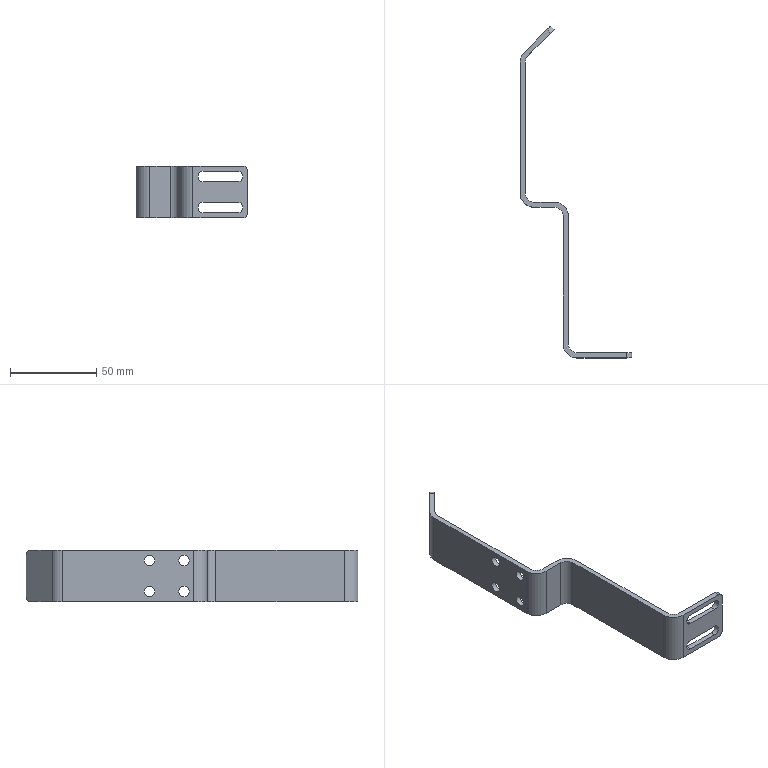Part | NX | features BREP 1 | 1 solid | 38 faces | box 65 x 192.678 x 30 mm | volume 21438 mm3 | cylinder 20 | plane 18 | commonest cylinder face diameters 6 x12 10 x4 16 x4
STEP:
#1=CARTESIAN_POINT('',(3.,82.5,30.));
#2=VERTEX_POINT('',#1);
#3=CARTESIAN_POINT('',(3.,82.5,0.));
#4=VERTEX_POINT('',#3);
#5=CARTESIAN_POINT('',(3.,82.5,30.));
#6=DIRECTION('',(0.,0.,-1.));
#7=VECTOR('',#6,1000.);
#8=LINE('',#5,#7);
#9=EDGE_CURVE('',#2,#4,#8,.T.);
#10=ORIENTED_EDGE('',*,*,#9,.F.);
#11=CARTESIAN_POINT('',(3.,8.,30.));
#12=VERTEX_POINT('',#11);
#13=CARTESIAN_POINT('',(3.,0.,30.));
#14=DIRECTION('',(0.,1.,0.));
#15=VECTOR('',#14,1000.);
#16=LINE('',#13,#15);
#17=EDGE_CURVE('',#12,#2,#16,.T.);
#18=ORIENTED_EDGE('',*,*,#17,.F.);
#19=CARTESIAN_POINT('',(3.,8.,0.));
#20=VERTEX_POINT('',#19);
#21=CARTESIAN_POINT('',(3.,8.,30.));
#22=DIRECTION('',(0.,0.,1.));
#23=VECTOR('',#22,1000.);
#24=LINE('',#21,#23);
#25=EDGE_CURVE('',#20,#12,#24,.T.);
#26=ORIENTED_EDGE('',*,*,#25,.F.);
#27=CARTESIAN_POINT('',(3.,0.,0.));
#28=DIRECTION('',(0.,-1.,0.));
#29=VECTOR('',#28,1000.);
#30=LINE('',#27,#29);
#31=EDGE_CURVE('',#4,#20,#30,.T.);
#32=ORIENTED_EDGE('',*,*,#31,.F.);
#33=EDGE_LOOP('',(#10,#18,#26,#32));
#34=FACE_BOUND('',#33,.T.);
#35=CARTESIAN_POINT('',(3.,0.,30.));
#36=DIRECTION('',(-1.,0.,0.));
#37=DIRECTION('',(0.,0.,-1.));
#38=AXIS2_PLACEMENT_3D('',#35,#36,#37);
#39=PLANE('',#38);
#40=ADVANCED_FACE('',(#34),#39,.F.);
#41=ORIENTED_EDGE('',*,*,#31,.T.);
#42=CARTESIAN_POINT('',(8.,3.,0.));
#43=VERTEX_POINT('',#42);
#44=CARTESIAN_POINT('',(8.,8.,0.));
#45=DIRECTION('',(0.,0.,1.));
#46=DIRECTION('',(-1.,0.,0.));
#47=AXIS2_PLACEMENT_3D('',#44,#45,#46);
#48=CIRCLE('',#47,5.);
#49=EDGE_CURVE('',#20,#43,#48,.T.);
#50=ORIENTED_EDGE('',*,*,#49,.T.);
#51=CARTESIAN_POINT('',(37.,3.,0.));
#52=VERTEX_POINT('',#51);
#53=CARTESIAN_POINT('',(40.,3.,0.));
#54=DIRECTION('',(1.,0.,0.));
#55=VECTOR('',#54,1000.);
#56=LINE('',#53,#55);
#57=EDGE_CURVE('',#43,#52,#56,.T.);
#58=ORIENTED_EDGE('',*,*,#57,.T.);
#59=CARTESIAN_POINT('',(37.,0.,0.));
#60=VERTEX_POINT('',#59);
#61=CARTESIAN_POINT('',(37.,8.,0.));
#62=DIRECTION('',(0.,-1.,0.));
#63=VECTOR('',#62,1000.);
#64=LINE('',#61,#63);
#65=EDGE_CURVE('',#52,#60,#64,.T.);
#66=ORIENTED_EDGE('',*,*,#65,.T.);
#67=CARTESIAN_POINT('',(8.,0.,0.));
#68=VERTEX_POINT('',#67);
#69=CARTESIAN_POINT('',(3.,0.,0.));
#70=DIRECTION('',(-1.,0.,0.));
#71=VECTOR('',#70,1000.);
#72=LINE('',#69,#71);
#73=EDGE_CURVE('',#60,#68,#72,.T.);
#74=ORIENTED_EDGE('',*,*,#73,.T.);
#75=CARTESIAN_POINT('',(0.,8.,0.));
#76=VERTEX_POINT('',#75);
#77=CARTESIAN_POINT('',(8.,8.,0.));
#78=DIRECTION('',(0.,0.,-1.));
#79=DIRECTION('',(-1.,0.,0.));
#80=AXIS2_PLACEMENT_3D('',#77,#78,#79);
#81=CIRCLE('',#80,8.);
#82=EDGE_CURVE('',#68,#76,#81,.T.);
#83=ORIENTED_EDGE('',*,*,#82,.T.);
#84=CARTESIAN_POINT('',(0.,82.5,0.));
#85=VERTEX_POINT('',#84);
#86=CARTESIAN_POINT('',(0.,90.5,0.));
#87=DIRECTION('',(0.,1.,0.));
#88=VECTOR('',#87,1000.);
#89=LINE('',#86,#88);
#90=EDGE_CURVE('',#76,#85,#89,.T.);
#91=ORIENTED_EDGE('',*,*,#90,.T.);
#92=CARTESIAN_POINT('',(-5.,87.5,0.));
#93=VERTEX_POINT('',#92);
#94=CARTESIAN_POINT('',(-5.,82.5,0.));
#95=DIRECTION('',(0.,0.,1.));
#96=DIRECTION('',(-1.,0.,0.));
#97=AXIS2_PLACEMENT_3D('',#94,#95,#96);
#98=CIRCLE('',#97,5.);
#99=EDGE_CURVE('',#85,#93,#98,.T.);
#100=ORIENTED_EDGE('',*,*,#99,.T.);
#101=CARTESIAN_POINT('',(-17.,87.5,0.));
#102=VERTEX_POINT('',#101);
#103=CARTESIAN_POINT('',(-22.,87.5,0.));
#104=DIRECTION('',(-1.,0.,0.));
#105=VECTOR('',#104,1000.);
#106=LINE('',#103,#105);
#107=EDGE_CURVE('',#93,#102,#106,.T.);
#108=ORIENTED_EDGE('',*,*,#107,.T.);
#109=CARTESIAN_POINT('',(-25.,95.5,0.));
#110=VERTEX_POINT('',#109);
#111=CARTESIAN_POINT('',(-17.,95.5,0.));
#112=DIRECTION('',(0.,0.,-1.));
#113=DIRECTION('',(-1.,0.,0.));
#114=AXIS2_PLACEMENT_3D('',#111,#112,#113);
#115=CIRCLE('',#114,8.);
#116=EDGE_CURVE('',#102,#110,#115,.T.);
#117=ORIENTED_EDGE('',*,*,#116,.T.);
#118=CARTESIAN_POINT('',(-25.,171.686,0.));
#119=VERTEX_POINT('',#118);
#120=CARTESIAN_POINT('',(-25.,175.222,0.));
#121=DIRECTION('',(0.,1.,0.));
#122=VECTOR('',#121,1000.);
#123=LINE('',#120,#122);
#124=EDGE_CURVE('',#110,#119,#123,.T.);
#125=ORIENTED_EDGE('',*,*,#124,.T.);
#126=CARTESIAN_POINT('',(-22.657,177.343,0.));
#127=VERTEX_POINT('',#126);
#128=CARTESIAN_POINT('',(-17.,171.686,0.));
#129=DIRECTION('',(0.,0.,-1.));
#130=DIRECTION('',(-1.,0.,0.));
#131=AXIS2_PLACEMENT_3D('',#128,#129,#130);
#132=CIRCLE('',#131,8.);
#133=EDGE_CURVE('',#119,#127,#132,.T.);
#134=ORIENTED_EDGE('',*,*,#133,.T.);
#135=CARTESIAN_POINT('',(-9.444,190.556,0.));
#136=VERTEX_POINT('',#135);
#137=CARTESIAN_POINT('',(-9.444,190.556,0.));
#138=DIRECTION('',(-0.7071,-0.7071,0.));
#139=VECTOR('',#138,1000.);
#140=LINE('',#137,#139);
#141=EDGE_CURVE('',#136,#127,#140,.T.);
#142=ORIENTED_EDGE('',*,*,#141,.F.);
#143=CARTESIAN_POINT('',(-7.322,188.435,0.));
#144=VERTEX_POINT('',#143);
#145=CARTESIAN_POINT('',(-7.322,188.435,0.));
#146=DIRECTION('',(-0.7071,0.7071,0.));
#147=VECTOR('',#146,1000.);
#148=LINE('',#145,#147);
#149=EDGE_CURVE('',#144,#136,#148,.T.);
#150=ORIENTED_EDGE('',*,*,#149,.F.);
#151=CARTESIAN_POINT('',(-20.536,175.222,0.));
#152=VERTEX_POINT('',#151);
#153=CARTESIAN_POINT('',(-22.879,172.879,0.));
#154=DIRECTION('',(-0.7071,-0.7071,0.));
#155=VECTOR('',#154,1000.);
#156=LINE('',#153,#155);
#157=EDGE_CURVE('',#144,#152,#156,.T.);
#158=ORIENTED_EDGE('',*,*,#157,.T.);
#159=CARTESIAN_POINT('',(-22.,171.686,0.));
#160=VERTEX_POINT('',#159);
#161=CARTESIAN_POINT('',(-17.,171.686,0.));
#162=DIRECTION('',(0.,0.,1.));
#163=DIRECTION('',(-1.,0.,0.));
#164=AXIS2_PLACEMENT_3D('',#161,#162,#163);
#165=CIRCLE('',#164,5.);
#166=EDGE_CURVE('',#152,#160,#165,.T.);
#167=ORIENTED_EDGE('',*,*,#166,.T.);
#168=CARTESIAN_POINT('',(-22.,95.5,0.));
#169=VERTEX_POINT('',#168);
#170=CARTESIAN_POINT('',(-22.,87.5,0.));
#171=DIRECTION('',(0.,-1.,0.));
#172=VECTOR('',#171,1000.);
#173=LINE('',#170,#172);
#174=EDGE_CURVE('',#160,#169,#173,.T.);
#175=ORIENTED_EDGE('',*,*,#174,.T.);
#176=CARTESIAN_POINT('',(-17.,90.5,0.));
#177=VERTEX_POINT('',#176);
#178=CARTESIAN_POINT('',(-17.,95.5,0.));
#179=DIRECTION('',(0.,0.,1.));
#180=DIRECTION('',(-1.,0.,0.));
#181=AXIS2_PLACEMENT_3D('',#178,#179,#180);
#182=CIRCLE('',#181,5.);
#183=EDGE_CURVE('',#169,#177,#182,.T.);
#184=ORIENTED_EDGE('',*,*,#183,.T.);
#185=CARTESIAN_POINT('',(-5.,90.5,0.));
#186=VERTEX_POINT('',#185);
#187=CARTESIAN_POINT('',(0.,90.5,0.));
#188=DIRECTION('',(1.,0.,0.));
#189=VECTOR('',#188,1000.);
#190=LINE('',#187,#189);
#191=EDGE_CURVE('',#177,#186,#190,.T.);
#192=ORIENTED_EDGE('',*,*,#191,.T.);
#193=CARTESIAN_POINT('',(-5.,82.5,0.));
#194=DIRECTION('',(0.,0.,1.));
#195=DIRECTION('',(-1.,0.,0.));
#196=AXIS2_PLACEMENT_3D('',#193,#194,#195);
#197=CIRCLE('',#196,8.);
#198=EDGE_CURVE('',#4,#186,#197,.T.);
#199=ORIENTED_EDGE('',*,*,#198,.F.);
#200=EDGE_LOOP('',(#41,#50,#58,#66,#74,#83,#91,#100,#108,#117,#125,#134,#142,#150,#158,#167,#175,#184,#192,#199));
#201=FACE_BOUND('',#200,.T.);
#202=CARTESIAN_POINT('',(-5.,90.5,0.));
#203=DIRECTION('',(0.,0.,-1.));
#204=DIRECTION('',(1.,0.,0.));
#205=AXIS2_PLACEMENT_3D('',#202,#203,#204);
#206=PLANE('',#205);
#207=ADVANCED_FACE('',(#201),#206,.T.);
#208=CARTESIAN_POINT('',(-5.,90.5,30.));
#209=VERTEX_POINT('',#208);
#210=CARTESIAN_POINT('',(-5.,82.5,30.));
#211=DIRECTION('',(0.,0.,-1.));
#212=DIRECTION('',(-1.,0.,0.));
#213=AXIS2_PLACEMENT_3D('',#210,#211,#212);
#214=CIRCLE('',#213,8.);
#215=EDGE_CURVE('',#209,#2,#214,.T.);
#216=ORIENTED_EDGE('',*,*,#215,.T.);
#217=ORIENTED_EDGE('',*,*,#9,.T.);
#218=ORIENTED_EDGE('',*,*,#198,.T.);
#219=CARTESIAN_POINT('',(-5.,90.5,30.));
#220=DIRECTION('',(0.,0.,1.));
#221=VECTOR('',#220,1000.);
#222=LINE('',#219,#221);
#223=EDGE_CURVE('',#186,#209,#222,.T.);
#224=ORIENTED_EDGE('',*,*,#223,.T.);
#225=EDGE_LOOP('',(#216,#217,#218,#224));
#226=FACE_BOUND('',#225,.T.);
#227=CARTESIAN_POINT('',(-5.,82.5,30.));
#228=DIRECTION('',(0.,0.,-1.));
#229=DIRECTION('',(1.,0.,0.));
#230=AXIS2_PLACEMENT_3D('',#227,#228,#229);
#231=CYLINDRICAL_SURFACE('',#230,8.);
#232=ADVANCED_FACE('',(#226),#231,.T.);
#233=ORIENTED_EDGE('',*,*,#17,.T.);
#234=ORIENTED_EDGE('',*,*,#215,.F.);
#235=CARTESIAN_POINT('',(-17.,90.5,30.));
#236=VERTEX_POINT('',#235);
#237=CARTESIAN_POINT('',(0.,90.5,30.));
#238=DIRECTION('',(-1.,0.,0.));
#239=VECTOR('',#238,1000.);
#240=LINE('',#237,#239);
#241=EDGE_CURVE('',#209,#236,#240,.T.);
#242=ORIENTED_EDGE('',*,*,#241,.T.);
#243=CARTESIAN_POINT('',(-22.,95.5,30.));
#244=VERTEX_POINT('',#243);
#245=CARTESIAN_POINT('',(-17.,95.5,30.));
#246=DIRECTION('',(0.,0.,-1.));
#247=DIRECTION('',(-1.,0.,0.));
#248=AXIS2_PLACEMENT_3D('',#245,#246,#247);
#249=CIRCLE('',#248,5.);
#250=EDGE_CURVE('',#236,#244,#249,.T.);
#251=ORIENTED_EDGE('',*,*,#250,.T.);
#252=CARTESIAN_POINT('',(-22.,171.686,30.));
#253=VERTEX_POINT('',#252);
#254=CARTESIAN_POINT('',(-22.,87.5,30.));
#255=DIRECTION('',(0.,1.,0.));
#256=VECTOR('',#255,1000.);
#257=LINE('',#254,#256);
#258=EDGE_CURVE('',#244,#253,#257,.T.);
#259=ORIENTED_EDGE('',*,*,#258,.T.);
#260=CARTESIAN_POINT('',(-20.536,175.222,30.));
#261=VERTEX_POINT('',#260);
#262=CARTESIAN_POINT('',(-17.,171.686,30.));
#263=DIRECTION('',(0.,0.,-1.));
#264=DIRECTION('',(-1.,0.,0.));
#265=AXIS2_PLACEMENT_3D('',#262,#263,#264);
#266=CIRCLE('',#265,5.);
#267=EDGE_CURVE('',#253,#261,#266,.T.);
#268=ORIENTED_EDGE('',*,*,#267,.T.);
#269=CARTESIAN_POINT('',(-7.322,188.435,30.));
#270=VERTEX_POINT('',#269);
#271=CARTESIAN_POINT('',(-22.879,172.879,30.));
#272=DIRECTION('',(0.7071,0.7071,0.));
#273=VECTOR('',#272,1000.);
#274=LINE('',#271,#273);
#275=EDGE_CURVE('',#261,#270,#274,.T.);
#276=ORIENTED_EDGE('',*,*,#275,.T.);
#277=CARTESIAN_POINT('',(-9.444,190.556,30.));
#278=VERTEX_POINT('',#277);
#279=CARTESIAN_POINT('',(-7.322,188.435,30.));
#280=DIRECTION('',(-0.7071,0.7071,0.));
#281=VECTOR('',#280,1000.);
#282=LINE('',#279,#281);
#283=EDGE_CURVE('',#270,#278,#282,.T.);
#284=ORIENTED_EDGE('',*,*,#283,.T.);
#285=CARTESIAN_POINT('',(-22.657,177.343,30.));
#286=VERTEX_POINT('',#285);
#287=CARTESIAN_POINT('',(-9.444,190.556,30.));
#288=DIRECTION('',(-0.7071,-0.7071,0.));
#289=VECTOR('',#288,1000.);
#290=LINE('',#287,#289);
#291=EDGE_CURVE('',#278,#286,#290,.T.);
#292=ORIENTED_EDGE('',*,*,#291,.T.);
#293=CARTESIAN_POINT('',(-25.,171.686,30.));
#294=VERTEX_POINT('',#293);
#295=CARTESIAN_POINT('',(-17.,171.686,30.));
#296=DIRECTION('',(0.,0.,1.));
#297=DIRECTION('',(-1.,0.,0.));
#298=AXIS2_PLACEMENT_3D('',#295,#296,#297);
#299=CIRCLE('',#298,8.);
#300=EDGE_CURVE('',#286,#294,#299,.T.);
#301=ORIENTED_EDGE('',*,*,#300,.T.);
#302=CARTESIAN_POINT('',(-25.,95.5,30.));
#303=VERTEX_POINT('',#302);
#304=CARTESIAN_POINT('',(-25.,90.5,30.));
#305=DIRECTION('',(0.,-1.,0.));
#306=VECTOR('',#305,1000.);
#307=LINE('',#304,#306);
#308=EDGE_CURVE('',#294,#303,#307,.T.);
#309=ORIENTED_EDGE('',*,*,#308,.T.);
#310=CARTESIAN_POINT('',(-17.,87.5,30.));
#311=VERTEX_POINT('',#310);
#312=CARTESIAN_POINT('',(-17.,95.5,30.));
#313=DIRECTION('',(0.,0.,1.));
#314=DIRECTION('',(-1.,0.,0.));
#315=AXIS2_PLACEMENT_3D('',#312,#313,#314);
#316=CIRCLE('',#315,8.);
#317=EDGE_CURVE('',#303,#311,#316,.T.);
#318=ORIENTED_EDGE('',*,*,#317,.T.);
#319=CARTESIAN_POINT('',(-5.,87.5,30.));
#320=VERTEX_POINT('',#319);
#321=CARTESIAN_POINT('',(3.,87.5,30.));
#322=DIRECTION('',(1.,0.,0.));
#323=VECTOR('',#322,1000.);
#324=LINE('',#321,#323);
#325=EDGE_CURVE('',#311,#320,#324,.T.);
#326=ORIENTED_EDGE('',*,*,#325,.T.);
#327=CARTESIAN_POINT('',(0.,82.5,30.));
#328=VERTEX_POINT('',#327);
#329=CARTESIAN_POINT('',(-5.,82.5,30.));
#330=DIRECTION('',(0.,0.,-1.));
#331=DIRECTION('',(-1.,0.,0.));
#332=AXIS2_PLACEMENT_3D('',#329,#330,#331);
#333=CIRCLE('',#332,5.);
#334=EDGE_CURVE('',#320,#328,#333,.T.);
#335=ORIENTED_EDGE('',*,*,#334,.T.);
#336=CARTESIAN_POINT('',(0.,8.,30.));
#337=VERTEX_POINT('',#336);
#338=CARTESIAN_POINT('',(0.,3.,30.));
#339=DIRECTION('',(0.,-1.,0.));
#340=VECTOR('',#339,1000.);
#341=LINE('',#338,#340);
#342=EDGE_CURVE('',#328,#337,#341,.T.);
#343=ORIENTED_EDGE('',*,*,#342,.T.);
#344=CARTESIAN_POINT('',(8.,0.,30.));
#345=VERTEX_POINT('',#344);
#346=CARTESIAN_POINT('',(8.,8.,30.));
#347=DIRECTION('',(0.,0.,1.));
#348=DIRECTION('',(-1.,0.,0.));
#349=AXIS2_PLACEMENT_3D('',#346,#347,#348);
#350=CIRCLE('',#349,8.);
#351=EDGE_CURVE('',#337,#345,#350,.T.);
#352=ORIENTED_EDGE('',*,*,#351,.T.);
#353=CARTESIAN_POINT('',(37.,0.,30.));
#354=VERTEX_POINT('',#353);
#355=CARTESIAN_POINT('',(-17.,0.,30.));
#356=DIRECTION('',(1.,0.,0.));
#357=VECTOR('',#356,1000.);
#358=LINE('',#355,#357);
#359=EDGE_CURVE('',#345,#354,#358,.T.);
#360=ORIENTED_EDGE('',*,*,#359,.T.);
#361=CARTESIAN_POINT('',(37.,3.,30.));
#362=VERTEX_POINT('',#361);
#363=CARTESIAN_POINT('',(37.,171.686,30.));
#364=DIRECTION('',(0.,1.,0.));
#365=VECTOR('',#364,1000.);
#366=LINE('',#363,#365);
#367=EDGE_CURVE('',#354,#362,#366,.T.);
#368=ORIENTED_EDGE('',*,*,#367,.T.);
#369=CARTESIAN_POINT('',(8.,3.,30.));
#370=VERTEX_POINT('',#369);
#371=CARTESIAN_POINT('',(40.,3.,30.));
#372=DIRECTION('',(-1.,0.,0.));
#373=VECTOR('',#372,1000.);
#374=LINE('',#371,#373);
#375=EDGE_CURVE('',#362,#370,#374,.T.);
#376=ORIENTED_EDGE('',*,*,#375,.T.);
#377=CARTESIAN_POINT('',(8.,8.,30.));
#378=DIRECTION('',(0.,0.,-1.));
#379=DIRECTION('',(-1.,0.,0.));
#380=AXIS2_PLACEMENT_3D('',#377,#378,#379);
#381=CIRCLE('',#380,5.);
#382=EDGE_CURVE('',#370,#12,#381,.T.);
#383=ORIENTED_EDGE('',*,*,#382,.T.);
#384=EDGE_LOOP('',(#233,#234,#242,#251,#259,#268,#276,#284,#292,#301,#309,#318,#326,#335,#343,#352,#360,#368,#376,#383));
#385=FACE_BOUND('',#384,.T.);
#386=CARTESIAN_POINT('',(8.,3.,30.));
#387=DIRECTION('',(0.,0.,1.));
#388=DIRECTION('',(-1.,0.,0.));
#389=AXIS2_PLACEMENT_3D('',#386,#387,#388);
#390=PLANE('',#389);
#391=ADVANCED_FACE('',(#385),#390,.T.);
#392=ORIENTED_EDGE('',*,*,#25,.T.);
#393=ORIENTED_EDGE('',*,*,#382,.F.);
#394=CARTESIAN_POINT('',(8.,3.,30.));
#395=DIRECTION('',(0.,0.,1.));
#396=VECTOR('',#395,1000.);
#397=LINE('',#394,#396);
#398=EDGE_CURVE('',#43,#370,#397,.T.);
#399=ORIENTED_EDGE('',*,*,#398,.F.);
#400=ORIENTED_EDGE('',*,*,#49,.F.);
#401=EDGE_LOOP('',(#392,#393,#399,#400));
#402=FACE_BOUND('',#401,.T.);
#403=CARTESIAN_POINT('',(8.,8.,30.));
#404=DIRECTION('',(0.,0.,-1.));
#405=DIRECTION('',(1.,0.,0.));
#406=AXIS2_PLACEMENT_3D('',#403,#404,#405);
#407=CYLINDRICAL_SURFACE('',#406,5.);
#408=ADVANCED_FACE('',(#402),#407,.F.);
#409=ORIENTED_EDGE('',*,*,#342,.F.);
#410=CARTESIAN_POINT('',(0.,82.5,30.));
#411=DIRECTION('',(0.,0.,-1.));
#412=VECTOR('',#411,1000.);
#413=LINE('',#410,#412);
#414=EDGE_CURVE('',#328,#85,#413,.T.);
#415=ORIENTED_EDGE('',*,*,#414,.T.);
#416=ORIENTED_EDGE('',*,*,#90,.F.);
#417=CARTESIAN_POINT('',(0.,8.,30.));
#418=DIRECTION('',(0.,0.,1.));
#419=VECTOR('',#418,1000.);
#420=LINE('',#417,#419);
#421=EDGE_CURVE('',#76,#337,#420,.T.);
#422=ORIENTED_EDGE('',*,*,#421,.T.);
#423=EDGE_LOOP('',(#409,#415,#416,#422));
#424=FACE_BOUND('',#423,.T.);
#425=CARTESIAN_POINT('',(0.,0.,30.));
#426=DIRECTION('',(-1.,0.,0.));
#427=DIRECTION('',(0.,0.,-1.));
#428=AXIS2_PLACEMENT_3D('',#425,#426,#427);
#429=PLANE('',#428);
#430=ADVANCED_FACE('',(#424),#429,.T.);
#431=CARTESIAN_POINT('',(-17.,90.5,30.));
#432=DIRECTION('',(0.,0.,-1.));
#433=VECTOR('',#432,1000.);
#434=LINE('',#431,#433);
#435=EDGE_CURVE('',#236,#177,#434,.T.);
#436=ORIENTED_EDGE('',*,*,#435,.F.);
#437=ORIENTED_EDGE('',*,*,#241,.F.);
#438=ORIENTED_EDGE('',*,*,#223,.F.);
#439=ORIENTED_EDGE('',*,*,#191,.F.);
#440=EDGE_LOOP('',(#436,#437,#438,#439));
#441=FACE_BOUND('',#440,.T.);
#442=CARTESIAN_POINT('',(0.,90.5,30.));
#443=DIRECTION('',(0.,-1.,0.));
#444=DIRECTION('',(0.,0.,1.));
#445=AXIS2_PLACEMENT_3D('',#442,#443,#444);
#446=PLANE('',#445);
#447=ADVANCED_FACE('',(#441),#446,.F.);
#448=CARTESIAN_POINT('',(40.,3.,27.));
#449=VERTEX_POINT('',#448);
#450=CARTESIAN_POINT('',(37.,3.,27.));
#451=DIRECTION('',(0.,-1.,0.));
#452=DIRECTION('',(0.,0.,-1.));
#453=AXIS2_PLACEMENT_3D('',#450,#451,#452);
#454=CIRCLE('',#453,3.);
#455=EDGE_CURVE('',#449,#362,#454,.T.);
#456=ORIENTED_EDGE('',*,*,#455,.F.);
#457=CARTESIAN_POINT('',(40.,3.,3.));
#458=VERTEX_POINT('',#457);
#459=CARTESIAN_POINT('',(40.,3.,30.));
#460=DIRECTION('',(0.,0.,1.));
#461=VECTOR('',#460,1000.);
#462=LINE('',#459,#461);
#463=EDGE_CURVE('',#458,#449,#462,.T.);
#464=ORIENTED_EDGE('',*,*,#463,.F.);
#465=CARTESIAN_POINT('',(37.,3.,3.));
#466=DIRECTION('',(0.,-1.,0.));
#467=DIRECTION('',(0.,0.,-1.));
#468=AXIS2_PLACEMENT_3D('',#465,#466,#467);
#469=CIRCLE('',#468,3.);
#470=EDGE_CURVE('',#52,#458,#469,.T.);
#471=ORIENTED_EDGE('',*,*,#470,.F.);
#472=ORIENTED_EDGE('',*,*,#57,.F.);
#473=ORIENTED_EDGE('',*,*,#398,.T.);
#474=ORIENTED_EDGE('',*,*,#375,.F.);
#475=EDGE_LOOP('',(#456,#464,#471,#472,#473,#474));
#476=FACE_BOUND('',#475,.T.);
#477=CARTESIAN_POINT('',(14.,3.,3.));
#478=VERTEX_POINT('',#477);
#479=CARTESIAN_POINT('',(14.,3.,9.));
#480=VERTEX_POINT('',#479);
#481=CARTESIAN_POINT('',(14.,3.,6.));
#482=DIRECTION('',(0.,1.,0.));
#483=DIRECTION('',(1.,0.,0.));
#484=AXIS2_PLACEMENT_3D('',#481,#482,#483);
#485=CIRCLE('',#484,3.);
#486=EDGE_CURVE('',#478,#480,#485,.T.);
#487=ORIENTED_EDGE('',*,*,#486,.F.);
#488=CARTESIAN_POINT('',(34.,3.,3.));
#489=VERTEX_POINT('',#488);
#490=CARTESIAN_POINT('',(40.,3.,3.));
#491=DIRECTION('',(-1.,0.,0.));
#492=VECTOR('',#491,1000.);
#493=LINE('',#490,#492);
#494=EDGE_CURVE('',#489,#478,#493,.T.);
#495=ORIENTED_EDGE('',*,*,#494,.F.);
#496=CARTESIAN_POINT('',(34.,3.,9.));
#497=VERTEX_POINT('',#496);
#498=CARTESIAN_POINT('',(34.,3.,6.));
#499=DIRECTION('',(0.,1.,0.));
#500=DIRECTION('',(1.,0.,0.));
#501=AXIS2_PLACEMENT_3D('',#498,#499,#500);
#502=CIRCLE('',#501,3.);
#503=EDGE_CURVE('',#497,#489,#502,.T.);
#504=ORIENTED_EDGE('',*,*,#503,.F.);
#505=CARTESIAN_POINT('',(40.,3.,9.));
#506=DIRECTION('',(1.,0.,0.));
#507=VECTOR('',#506,1000.);
#508=LINE('',#505,#507);
#509=EDGE_CURVE('',#480,#497,#508,.T.);
#510=ORIENTED_EDGE('',*,*,#509,.F.);
#511=EDGE_LOOP('',(#487,#495,#504,#510));
#512=FACE_BOUND('',#511,.T.);
#513=CARTESIAN_POINT('',(14.,3.,21.));
#514=VERTEX_POINT('',#513);
#515=CARTESIAN_POINT('',(14.,3.,27.));
#516=VERTEX_POINT('',#515);
#517=CARTESIAN_POINT('',(14.,3.,24.));
#518=DIRECTION('',(0.,1.,0.));
#519=DIRECTION('',(1.,0.,0.));
#520=AXIS2_PLACEMENT_3D('',#517,#518,#519);
#521=CIRCLE('',#520,3.);
#522=EDGE_CURVE('',#514,#516,#521,.T.);
#523=ORIENTED_EDGE('',*,*,#522,.F.);
#524=CARTESIAN_POINT('',(34.,3.,21.));
#525=VERTEX_POINT('',#524);
#526=CARTESIAN_POINT('',(40.,3.,21.));
#527=DIRECTION('',(-1.,0.,0.));
#528=VECTOR('',#527,1000.);
#529=LINE('',#526,#528);
#530=EDGE_CURVE('',#525,#514,#529,.T.);
#531=ORIENTED_EDGE('',*,*,#530,.F.);
#532=CARTESIAN_POINT('',(34.,3.,27.));
#533=VERTEX_POINT('',#532);
#534=CARTESIAN_POINT('',(34.,3.,24.));
#535=DIRECTION('',(0.,1.,0.));
#536=DIRECTION('',(1.,0.,0.));
#537=AXIS2_PLACEMENT_3D('',#534,#535,#536);
#538=CIRCLE('',#537,3.);
#539=EDGE_CURVE('',#533,#525,#538,.T.);
#540=ORIENTED_EDGE('',*,*,#539,.F.);
#541=CARTESIAN_POINT('',(40.,3.,27.));
#542=DIRECTION('',(1.,0.,0.));
#543=VECTOR('',#542,1000.);
#544=LINE('',#541,#543);
#545=EDGE_CURVE('',#516,#533,#544,.T.);
#546=ORIENTED_EDGE('',*,*,#545,.F.);
#547=EDGE_LOOP('',(#523,#531,#540,#546));
#548=FACE_BOUND('',#547,.T.);
#549=CARTESIAN_POINT('',(40.,3.,30.));
#550=DIRECTION('',(0.,-1.,0.));
#551=DIRECTION('',(-1.,0.,0.));
#552=AXIS2_PLACEMENT_3D('',#549,#550,#551);
#553=PLANE('',#552);
#554=ADVANCED_FACE('',(#476,#512,#548),#553,.F.);
#555=ORIENTED_EDGE('',*,*,#351,.F.);
#556=ORIENTED_EDGE('',*,*,#421,.F.);
#557=ORIENTED_EDGE('',*,*,#82,.F.);
#558=CARTESIAN_POINT('',(8.,0.,30.));
#559=DIRECTION('',(0.,0.,1.));
#560=VECTOR('',#559,1000.);
#561=LINE('',#558,#560);
#562=EDGE_CURVE('',#68,#345,#561,.T.);
#563=ORIENTED_EDGE('',*,*,#562,.T.);
#564=EDGE_LOOP('',(#555,#556,#557,#563));
#565=FACE_BOUND('',#564,.T.);
#566=CARTESIAN_POINT('',(8.,8.,30.));
#567=DIRECTION('',(0.,0.,-1.));
#568=DIRECTION('',(1.,0.,0.));
#569=AXIS2_PLACEMENT_3D('',#566,#567,#568);
#570=CYLINDRICAL_SURFACE('',#569,8.);
#571=ADVANCED_FACE('',(#565),#570,.T.);
#572=ORIENTED_EDGE('',*,*,#414,.F.);
#573=ORIENTED_EDGE('',*,*,#334,.F.);
#574=CARTESIAN_POINT('',(-5.,87.5,30.));
#575=DIRECTION('',(0.,0.,1.));
#576=VECTOR('',#575,1000.);
#577=LINE('',#574,#576);
#578=EDGE_CURVE('',#93,#320,#577,.T.);
#579=ORIENTED_EDGE('',*,*,#578,.F.);
#580=ORIENTED_EDGE('',*,*,#99,.F.);
#581=EDGE_LOOP('',(#572,#573,#579,#580));
#582=FACE_BOUND('',#581,.T.);
#583=CARTESIAN_POINT('',(-5.,82.5,30.));
#584=DIRECTION('',(0.,0.,-1.));
#585=DIRECTION('',(1.,0.,0.));
#586=AXIS2_PLACEMENT_3D('',#583,#584,#585);
#587=CYLINDRICAL_SURFACE('',#586,5.);
#588=ADVANCED_FACE('',(#582),#587,.F.);
#589=CARTESIAN_POINT('',(-22.,95.5,30.));
#590=DIRECTION('',(0.,0.,-1.));
#591=VECTOR('',#590,1000.);
#592=LINE('',#589,#591);
#593=EDGE_CURVE('',#244,#169,#592,.T.);
#594=ORIENTED_EDGE('',*,*,#593,.F.);
#595=ORIENTED_EDGE('',*,*,#250,.F.);
#596=ORIENTED_EDGE('',*,*,#435,.T.);
#597=ORIENTED_EDGE('',*,*,#183,.F.);
#598=EDGE_LOOP('',(#594,#595,#596,#597));
#599=FACE_BOUND('',#598,.T.);
#600=CARTESIAN_POINT('',(-17.,95.5,30.));
#601=DIRECTION('',(0.,0.,-1.));
#602=DIRECTION('',(1.,0.,0.));
#603=AXIS2_PLACEMENT_3D('',#600,#601,#602);
#604=CYLINDRICAL_SURFACE('',#603,5.);
#605=ADVANCED_FACE('',(#599),#604,.F.);
#606=CARTESIAN_POINT('',(40.,0.,27.));
#607=VERTEX_POINT('',#606);
#608=CARTESIAN_POINT('',(37.,0.,27.));
#609=DIRECTION('',(0.,1.,0.));
#610=DIRECTION('',(0.,0.,-1.));
#611=AXIS2_PLACEMENT_3D('',#608,#609,#610);
#612=CIRCLE('',#611,3.);
#613=EDGE_CURVE('',#354,#607,#612,.T.);
#614=ORIENTED_EDGE('',*,*,#613,.T.);
#615=CARTESIAN_POINT('',(40.,3.,27.));
#616=DIRECTION('',(0.,1.,0.));
#617=VECTOR('',#616,1000.);
#618=LINE('',#615,#617);
#619=EDGE_CURVE('',#607,#449,#618,.T.);
#620=ORIENTED_EDGE('',*,*,#619,.T.);
#621=ORIENTED_EDGE('',*,*,#455,.T.);
#622=ORIENTED_EDGE('',*,*,#367,.F.);
#623=EDGE_LOOP('',(#614,#620,#621,#622));
#624=FACE_BOUND('',#623,.T.);
#625=CARTESIAN_POINT('',(37.,3.,27.));
#626=DIRECTION('',(0.,-1.,0.));
#627=DIRECTION('',(0.,0.,1.));
#628=AXIS2_PLACEMENT_3D('',#625,#626,#627);
#629=CYLINDRICAL_SURFACE('',#628,3.);
#630=ADVANCED_FACE('',(#624),#629,.T.);
#631=CARTESIAN_POINT('',(40.,0.,3.));
#632=VERTEX_POINT('',#631);
#633=CARTESIAN_POINT('',(40.,0.,30.));
#634=DIRECTION('',(0.,0.,-1.));
#635=VECTOR('',#634,1000.);
#636=LINE('',#633,#635);
#637=EDGE_CURVE('',#607,#632,#636,.T.);
#638=ORIENTED_EDGE('',*,*,#637,.T.);
#639=CARTESIAN_POINT('',(40.,3.,3.));
#640=DIRECTION('',(0.,1.,0.));
#641=VECTOR('',#640,1000.);
#642=LINE('',#639,#641);
#643=EDGE_CURVE('',#632,#458,#642,.T.);
#644=ORIENTED_EDGE('',*,*,#643,.T.);
#645=ORIENTED_EDGE('',*,*,#463,.T.);
#646=ORIENTED_EDGE('',*,*,#619,.F.);
#647=EDGE_LOOP('',(#638,#644,#645,#646));
#648=FACE_BOUND('',#647,.T.);
#649=CARTESIAN_POINT('',(40.,3.,30.));
#650=DIRECTION('',(1.,0.,0.));
#651=DIRECTION('',(0.,0.,1.));
#652=AXIS2_PLACEMENT_3D('',#649,#650,#651);
#653=PLANE('',#652);
#654=ADVANCED_FACE('',(#648),#653,.T.);
#655=CARTESIAN_POINT('',(37.,0.,3.));
#656=DIRECTION('',(0.,1.,0.));
#657=DIRECTION('',(0.,0.,-1.));
#658=AXIS2_PLACEMENT_3D('',#655,#656,#657);
#659=CIRCLE('',#658,3.);
#660=EDGE_CURVE('',#632,#60,#659,.T.);
#661=ORIENTED_EDGE('',*,*,#660,.T.);
#662=ORIENTED_EDGE('',*,*,#65,.F.);
#663=ORIENTED_EDGE('',*,*,#470,.T.);
#664=ORIENTED_EDGE('',*,*,#643,.F.);
#665=EDGE_LOOP('',(#661,#662,#663,#664));
#666=FACE_BOUND('',#665,.T.);
#667=CARTESIAN_POINT('',(37.,8.,3.));
#668=DIRECTION('',(0.,-1.,0.));
#669=DIRECTION('',(0.,0.,1.));
#670=AXIS2_PLACEMENT_3D('',#667,#668,#669);
#671=CYLINDRICAL_SURFACE('',#670,3.);
#672=ADVANCED_FACE('',(#666),#671,.T.);
#673=CARTESIAN_POINT('',(14.,0.,9.));
#674=VERTEX_POINT('',#673);
#675=CARTESIAN_POINT('',(34.,0.,9.));
#676=VERTEX_POINT('',#675);
#677=CARTESIAN_POINT('',(14.,0.,9.));
#678=DIRECTION('',(1.,0.,0.));
#679=VECTOR('',#678,1000.);
#680=LINE('',#677,#679);
#681=EDGE_CURVE('',#674,#676,#680,.T.);
#682=ORIENTED_EDGE('',*,*,#681,.F.);
#683=CARTESIAN_POINT('',(14.,10.,9.));
#684=DIRECTION('',(0.,-1.,0.));
#685=VECTOR('',#684,1000.);
#686=LINE('',#683,#685);
#687=EDGE_CURVE('',#480,#674,#686,.T.);
#688=ORIENTED_EDGE('',*,*,#687,.F.);
#689=ORIENTED_EDGE('',*,*,#509,.T.);
#690=CARTESIAN_POINT('',(34.,10.,9.));
#691=DIRECTION('',(0.,1.,0.));
#692=VECTOR('',#691,1000.);
#693=LINE('',#690,#692);
#694=EDGE_CURVE('',#676,#497,#693,.T.);
#695=ORIENTED_EDGE('',*,*,#694,.F.);
#696=EDGE_LOOP('',(#682,#688,#689,#695));
#697=FACE_BOUND('',#696,.T.);
#698=CARTESIAN_POINT('',(14.,10.,9.));
#699=DIRECTION('',(0.,0.,1.));
#700=DIRECTION('',(-1.,0.,0.));
#701=AXIS2_PLACEMENT_3D('',#698,#699,#700);
#702=PLANE('',#701);
#703=ADVANCED_FACE('',(#697),#702,.F.);
#704=CARTESIAN_POINT('',(14.,0.,3.));
#705=VERTEX_POINT('',#704);
#706=CARTESIAN_POINT('',(14.,0.,6.));
#707=DIRECTION('',(0.,1.,0.));
#708=DIRECTION('',(1.,0.,0.));
#709=AXIS2_PLACEMENT_3D('',#706,#707,#708);
#710=CIRCLE('',#709,3.);
#711=EDGE_CURVE('',#705,#674,#710,.T.);
#712=ORIENTED_EDGE('',*,*,#711,.F.);
#713=CARTESIAN_POINT('',(14.,10.,3.));
#714=DIRECTION('',(0.,-1.,0.));
#715=VECTOR('',#714,1000.);
#716=LINE('',#713,#715);
#717=EDGE_CURVE('',#478,#705,#716,.T.);
#718=ORIENTED_EDGE('',*,*,#717,.F.);
#719=ORIENTED_EDGE('',*,*,#486,.T.);
#720=ORIENTED_EDGE('',*,*,#687,.T.);
#721=EDGE_LOOP('',(#712,#718,#719,#720));
#722=FACE_BOUND('',#721,.T.);
#723=CARTESIAN_POINT('',(14.,10.,6.));
#724=DIRECTION('',(0.,-1.,0.));
#725=DIRECTION('',(-1.,0.,0.));
#726=AXIS2_PLACEMENT_3D('',#723,#724,#725);
#727=CYLINDRICAL_SURFACE('',#726,3.);
#728=ADVANCED_FACE('',(#722),#727,.F.);
#729=CARTESIAN_POINT('',(34.,0.,3.));
#730=VERTEX_POINT('',#729);
#731=CARTESIAN_POINT('',(14.,0.,3.));
#732=DIRECTION('',(-1.,0.,0.));
#733=VECTOR('',#732,1000.);
#734=LINE('',#731,#733);
#735=EDGE_CURVE('',#730,#705,#734,.T.);
#736=ORIENTED_EDGE('',*,*,#735,.F.);
#737=CARTESIAN_POINT('',(34.,10.,3.));
#738=DIRECTION('',(0.,-1.,0.));
#739=VECTOR('',#738,1000.);
#740=LINE('',#737,#739);
#741=EDGE_CURVE('',#489,#730,#740,.T.);
#742=ORIENTED_EDGE('',*,*,#741,.F.);
#743=ORIENTED_EDGE('',*,*,#494,.T.);
#744=ORIENTED_EDGE('',*,*,#717,.T.);
#745=EDGE_LOOP('',(#736,#742,#743,#744));
#746=FACE_BOUND('',#745,.T.);
#747=CARTESIAN_POINT('',(14.,10.,3.));
#748=DIRECTION('',(0.,0.,-1.));
#749=DIRECTION('',(1.,0.,0.));
#750=AXIS2_PLACEMENT_3D('',#747,#748,#749);
#751=PLANE('',#750);
#752=ADVANCED_FACE('',(#746),#751,.F.);
#753=ORIENTED_EDGE('',*,*,#503,.T.);
#754=ORIENTED_EDGE('',*,*,#741,.T.);
#755=CARTESIAN_POINT('',(34.,0.,6.));
#756=DIRECTION('',(0.,1.,0.));
#757=DIRECTION('',(1.,0.,0.));
#758=AXIS2_PLACEMENT_3D('',#755,#756,#757);
#759=CIRCLE('',#758,3.);
#760=EDGE_CURVE('',#676,#730,#759,.T.);
#761=ORIENTED_EDGE('',*,*,#760,.F.);
#762=ORIENTED_EDGE('',*,*,#694,.T.);
#763=EDGE_LOOP('',(#753,#754,#761,#762));
#764=FACE_BOUND('',#763,.T.);
#765=CARTESIAN_POINT('',(34.,10.,6.));
#766=DIRECTION('',(0.,-1.,0.));
#767=DIRECTION('',(-1.,0.,0.));
#768=AXIS2_PLACEMENT_3D('',#765,#766,#767);
#769=CYLINDRICAL_SURFACE('',#768,3.);
#770=ADVANCED_FACE('',(#764),#769,.F.);
#771=CARTESIAN_POINT('',(14.,0.,27.));
#772=VERTEX_POINT('',#771);
#773=CARTESIAN_POINT('',(34.,0.,27.));
#774=VERTEX_POINT('',#773);
#775=CARTESIAN_POINT('',(14.,0.,27.));
#776=DIRECTION('',(1.,0.,0.));
#777=VECTOR('',#776,1000.);
#778=LINE('',#775,#777);
#779=EDGE_CURVE('',#772,#774,#778,.T.);
#780=ORIENTED_EDGE('',*,*,#779,.F.);
#781=CARTESIAN_POINT('',(14.,10.,27.));
#782=DIRECTION('',(0.,-1.,0.));
#783=VECTOR('',#782,1000.);
#784=LINE('',#781,#783);
#785=EDGE_CURVE('',#516,#772,#784,.T.);
#786=ORIENTED_EDGE('',*,*,#785,.F.);
#787=ORIENTED_EDGE('',*,*,#545,.T.);
#788=CARTESIAN_POINT('',(34.,10.,27.));
#789=DIRECTION('',(0.,1.,0.));
#790=VECTOR('',#789,1000.);
#791=LINE('',#788,#790);
#792=EDGE_CURVE('',#774,#533,#791,.T.);
#793=ORIENTED_EDGE('',*,*,#792,.F.);
#794=EDGE_LOOP('',(#780,#786,#787,#793));
#795=FACE_BOUND('',#794,.T.);
#796=CARTESIAN_POINT('',(14.,10.,27.));
#797=DIRECTION('',(0.,0.,1.));
#798=DIRECTION('',(-1.,0.,0.));
#799=AXIS2_PLACEMENT_3D('',#796,#797,#798);
#800=PLANE('',#799);
#801=ADVANCED_FACE('',(#795),#800,.F.);
#802=CARTESIAN_POINT('',(14.,0.,21.));
#803=VERTEX_POINT('',#802);
#804=CARTESIAN_POINT('',(14.,0.,24.));
#805=DIRECTION('',(0.,1.,0.));
#806=DIRECTION('',(1.,0.,0.));
#807=AXIS2_PLACEMENT_3D('',#804,#805,#806);
#808=CIRCLE('',#807,3.);
#809=EDGE_CURVE('',#803,#772,#808,.T.);
#810=ORIENTED_EDGE('',*,*,#809,.F.);
#811=CARTESIAN_POINT('',(14.,10.,21.));
#812=DIRECTION('',(0.,-1.,0.));
#813=VECTOR('',#812,1000.);
#814=LINE('',#811,#813);
#815=EDGE_CURVE('',#514,#803,#814,.T.);
#816=ORIENTED_EDGE('',*,*,#815,.F.);
#817=ORIENTED_EDGE('',*,*,#522,.T.);
#818=ORIENTED_EDGE('',*,*,#785,.T.);
#819=EDGE_LOOP('',(#810,#816,#817,#818));
#820=FACE_BOUND('',#819,.T.);
#821=CARTESIAN_POINT('',(14.,10.,24.));
#822=DIRECTION('',(0.,-1.,0.));
#823=DIRECTION('',(-1.,0.,0.));
#824=AXIS2_PLACEMENT_3D('',#821,#822,#823);
#825=CYLINDRICAL_SURFACE('',#824,3.);
#826=ADVANCED_FACE('',(#820),#825,.F.);
#827=CARTESIAN_POINT('',(34.,0.,21.));
#828=VERTEX_POINT('',#827);
#829=CARTESIAN_POINT('',(14.,0.,21.));
#830=DIRECTION('',(-1.,0.,0.));
#831=VECTOR('',#830,1000.);
#832=LINE('',#829,#831);
#833=EDGE_CURVE('',#828,#803,#832,.T.);
#834=ORIENTED_EDGE('',*,*,#833,.F.);
#835=CARTESIAN_POINT('',(34.,10.,21.));
#836=DIRECTION('',(0.,-1.,0.));
#837=VECTOR('',#836,1000.);
#838=LINE('',#835,#837);
#839=EDGE_CURVE('',#525,#828,#838,.T.);
#840=ORIENTED_EDGE('',*,*,#839,.F.);
#841=ORIENTED_EDGE('',*,*,#530,.T.);
#842=ORIENTED_EDGE('',*,*,#815,.T.);
#843=EDGE_LOOP('',(#834,#840,#841,#842));
#844=FACE_BOUND('',#843,.T.);
#845=CARTESIAN_POINT('',(14.,10.,21.));
#846=DIRECTION('',(0.,0.,-1.));
#847=DIRECTION('',(1.,0.,0.));
#848=AXIS2_PLACEMENT_3D('',#845,#846,#847);
#849=PLANE('',#848);
#850=ADVANCED_FACE('',(#844),#849,.F.);
#851=ORIENTED_EDGE('',*,*,#539,.T.);
#852=ORIENTED_EDGE('',*,*,#839,.T.);
#853=CARTESIAN_POINT('',(34.,0.,24.));
#854=DIRECTION('',(0.,1.,0.));
#855=DIRECTION('',(1.,0.,0.));
#856=AXIS2_PLACEMENT_3D('',#853,#854,#855);
#857=CIRCLE('',#856,3.);
#858=EDGE_CURVE('',#774,#828,#857,.T.);
#859=ORIENTED_EDGE('',*,*,#858,.F.);
#860=ORIENTED_EDGE('',*,*,#792,.T.);
#861=EDGE_LOOP('',(#851,#852,#859,#860));
#862=FACE_BOUND('',#861,.T.);
#863=CARTESIAN_POINT('',(34.,10.,24.));
#864=DIRECTION('',(0.,-1.,0.));
#865=DIRECTION('',(-1.,0.,0.));
#866=AXIS2_PLACEMENT_3D('',#863,#864,#865);
#867=CYLINDRICAL_SURFACE('',#866,3.);
#868=ADVANCED_FACE('',(#862),#867,.F.);
#869=ORIENTED_EDGE('',*,*,#73,.F.);
#870=ORIENTED_EDGE('',*,*,#660,.F.);
#871=ORIENTED_EDGE('',*,*,#637,.F.);
#872=ORIENTED_EDGE('',*,*,#613,.F.);
#873=ORIENTED_EDGE('',*,*,#359,.F.);
#874=ORIENTED_EDGE('',*,*,#562,.F.);
#875=EDGE_LOOP('',(#869,#870,#871,#872,#873,#874));
#876=FACE_BOUND('',#875,.T.);
#877=ORIENTED_EDGE('',*,*,#760,.T.);
#878=ORIENTED_EDGE('',*,*,#735,.T.);
#879=ORIENTED_EDGE('',*,*,#711,.T.);
#880=ORIENTED_EDGE('',*,*,#681,.T.);
#881=EDGE_LOOP('',(#877,#878,#879,#880));
#882=FACE_BOUND('',#881,.T.);
#883=ORIENTED_EDGE('',*,*,#858,.T.);
#884=ORIENTED_EDGE('',*,*,#833,.T.);
#885=ORIENTED_EDGE('',*,*,#809,.T.);
#886=ORIENTED_EDGE('',*,*,#779,.T.);
#887=EDGE_LOOP('',(#883,#884,#885,#886));
#888=FACE_BOUND('',#887,.T.);
#889=CARTESIAN_POINT('',(40.,0.,30.));
#890=DIRECTION('',(0.,-1.,0.));
#891=DIRECTION('',(-1.,0.,0.));
#892=AXIS2_PLACEMENT_3D('',#889,#890,#891);
#893=PLANE('',#892);
#894=ADVANCED_FACE('',(#876,#882,#888),#893,.T.);
#895=ORIENTED_EDGE('',*,*,#325,.F.);
#896=CARTESIAN_POINT('',(-17.,87.5,30.));
#897=DIRECTION('',(0.,0.,-1.));
#898=VECTOR('',#897,1000.);
#899=LINE('',#896,#898);
#900=EDGE_CURVE('',#311,#102,#899,.T.);
#901=ORIENTED_EDGE('',*,*,#900,.T.);
#902=ORIENTED_EDGE('',*,*,#107,.F.);
#903=ORIENTED_EDGE('',*,*,#578,.T.);
#904=EDGE_LOOP('',(#895,#901,#902,#903));
#905=FACE_BOUND('',#904,.T.);
#906=CARTESIAN_POINT('',(0.,87.5,30.));
#907=DIRECTION('',(0.,-1.,0.));
#908=DIRECTION('',(0.,0.,1.));
#909=AXIS2_PLACEMENT_3D('',#906,#907,#908);
#910=PLANE('',#909);
#911=ADVANCED_FACE('',(#905),#910,.T.);
#912=CARTESIAN_POINT('',(-22.,171.686,30.));
#913=DIRECTION('',(0.,0.,-1.));
#914=VECTOR('',#913,1000.);
#915=LINE('',#912,#914);
#916=EDGE_CURVE('',#253,#160,#915,.T.);
#917=ORIENTED_EDGE('',*,*,#916,.F.);
#918=ORIENTED_EDGE('',*,*,#258,.F.);
#919=ORIENTED_EDGE('',*,*,#593,.T.);
#920=ORIENTED_EDGE('',*,*,#174,.F.);
#921=EDGE_LOOP('',(#917,#918,#919,#920));
#922=FACE_BOUND('',#921,.T.);
#923=CARTESIAN_POINT('',(-22.,101.,27.));
#924=VERTEX_POINT('',#923);
#925=CARTESIAN_POINT('',(-22.,101.,24.));
#926=DIRECTION('',(1.,0.,0.));
#927=DIRECTION('',(0.,0.,1.));
#928=AXIS2_PLACEMENT_3D('',#925,#926,#927);
#929=CIRCLE('',#928,3.);
#930=EDGE_CURVE('',#924,#924,#929,.T.);
#931=ORIENTED_EDGE('',*,*,#930,.F.);
#932=EDGE_LOOP('',(#931));
#933=FACE_BOUND('',#932,.T.);
#934=CARTESIAN_POINT('',(-22.,121.,27.));
#935=VERTEX_POINT('',#934);
#936=CARTESIAN_POINT('',(-22.,121.,24.));
#937=DIRECTION('',(1.,0.,0.));
#938=DIRECTION('',(0.,0.,1.));
#939=AXIS2_PLACEMENT_3D('',#936,#937,#938);
#940=CIRCLE('',#939,3.);
#941=EDGE_CURVE('',#935,#935,#940,.T.);
#942=ORIENTED_EDGE('',*,*,#941,.F.);
#943=EDGE_LOOP('',(#942));
#944=FACE_BOUND('',#943,.T.);
#945=CARTESIAN_POINT('',(-22.,101.,9.));
#946=VERTEX_POINT('',#945);
#947=CARTESIAN_POINT('',(-22.,101.,6.));
#948=DIRECTION('',(1.,0.,0.));
#949=DIRECTION('',(0.,0.,1.));
#950=AXIS2_PLACEMENT_3D('',#947,#948,#949);
#951=CIRCLE('',#950,3.);
#952=EDGE_CURVE('',#946,#946,#951,.T.);
#953=ORIENTED_EDGE('',*,*,#952,.F.);
#954=EDGE_LOOP('',(#953));
#955=FACE_BOUND('',#954,.T.);
#956=CARTESIAN_POINT('',(-22.,121.,9.));
#957=VERTEX_POINT('',#956);
#958=CARTESIAN_POINT('',(-22.,121.,6.));
#959=DIRECTION('',(1.,0.,0.));
#960=DIRECTION('',(0.,0.,1.));
#961=AXIS2_PLACEMENT_3D('',#958,#959,#960);
#962=CIRCLE('',#961,3.);
#963=EDGE_CURVE('',#957,#957,#962,.T.);
#964=ORIENTED_EDGE('',*,*,#963,.F.);
#965=EDGE_LOOP('',(#964));
#966=FACE_BOUND('',#965,.T.);
#967=CARTESIAN_POINT('',(-22.,87.5,30.));
#968=DIRECTION('',(-1.,0.,0.));
#969=DIRECTION('',(0.,1.,0.));
#970=AXIS2_PLACEMENT_3D('',#967,#968,#969);
#971=PLANE('',#970);
#972=ADVANCED_FACE('',(#922,#933,#944,#955,#966),#971,.F.);
#973=ORIENTED_EDGE('',*,*,#317,.F.);
#974=CARTESIAN_POINT('',(-25.,95.5,30.));
#975=DIRECTION('',(0.,0.,-1.));
#976=VECTOR('',#975,1000.);
#977=LINE('',#974,#976);
#978=EDGE_CURVE('',#303,#110,#977,.T.);
#979=ORIENTED_EDGE('',*,*,#978,.T.);
#980=ORIENTED_EDGE('',*,*,#116,.F.);
#981=ORIENTED_EDGE('',*,*,#900,.F.);
#982=EDGE_LOOP('',(#973,#979,#980,#981));
#983=FACE_BOUND('',#982,.T.);
#984=CARTESIAN_POINT('',(-17.,95.5,30.));
#985=DIRECTION('',(0.,0.,-1.));
#986=DIRECTION('',(1.,0.,0.));
#987=AXIS2_PLACEMENT_3D('',#984,#985,#986);
#988=CYLINDRICAL_SURFACE('',#987,8.);
#989=ADVANCED_FACE('',(#983),#988,.T.);
#990=CARTESIAN_POINT('',(-20.536,175.222,30.));
#991=DIRECTION('',(0.,0.,-1.));
#992=VECTOR('',#991,1000.);
#993=LINE('',#990,#992);
#994=EDGE_CURVE('',#261,#152,#993,.T.);
#995=ORIENTED_EDGE('',*,*,#994,.F.);
#996=ORIENTED_EDGE('',*,*,#267,.F.);
#997=ORIENTED_EDGE('',*,*,#916,.T.);
#998=ORIENTED_EDGE('',*,*,#166,.F.);
#999=EDGE_LOOP('',(#995,#996,#997,#998));
#1000=FACE_BOUND('',#999,.T.);
#1001=CARTESIAN_POINT('',(-17.,171.686,30.));
#1002=DIRECTION('',(0.,0.,-1.));
#1003=DIRECTION('',(1.,0.,0.));
#1004=AXIS2_PLACEMENT_3D('',#1001,#1002,#1003);
#1005=CYLINDRICAL_SURFACE('',#1004,5.);
#1006=ADVANCED_FACE('',(#1000),#1005,.F.);
#1007=ORIENTED_EDGE('',*,*,#930,.T.);
#1008=EDGE_LOOP('',(#1007));
#1009=FACE_BOUND('',#1008,.T.);
#1010=CARTESIAN_POINT('',(-25.,101.,27.));
#1011=VERTEX_POINT('',#1010);
#1012=CARTESIAN_POINT('',(-25.,101.,24.));
#1013=DIRECTION('',(1.,0.,0.));
#1014=DIRECTION('',(0.,0.,1.));
#1015=AXIS2_PLACEMENT_3D('',#1012,#1013,#1014);
#1016=CIRCLE('',#1015,3.);
#1017=EDGE_CURVE('',#1011,#1011,#1016,.T.);
#1018=ORIENTED_EDGE('',*,*,#1017,.F.);
#1019=EDGE_LOOP('',(#1018));
#1020=FACE_BOUND('',#1019,.T.);
#1021=CARTESIAN_POINT('',(-25.,101.,24.));
#1022=DIRECTION('',(-1.,0.,0.));
#1023=DIRECTION('',(0.,0.,-1.));
#1024=AXIS2_PLACEMENT_3D('',#1021,#1022,#1023);
#1025=CYLINDRICAL_SURFACE('',#1024,3.);
#1026=ADVANCED_FACE('',(#1009,#1020),#1025,.F.);
#1027=ORIENTED_EDGE('',*,*,#941,.T.);
#1028=EDGE_LOOP('',(#1027));
#1029=FACE_BOUND('',#1028,.T.);
#1030=CARTESIAN_POINT('',(-25.,121.,27.));
#1031=VERTEX_POINT('',#1030);
#1032=CARTESIAN_POINT('',(-25.,121.,24.));
#1033=DIRECTION('',(1.,0.,0.));
#1034=DIRECTION('',(0.,0.,1.));
#1035=AXIS2_PLACEMENT_3D('',#1032,#1033,#1034);
#1036=CIRCLE('',#1035,3.);
#1037=EDGE_CURVE('',#1031,#1031,#1036,.T.);
#1038=ORIENTED_EDGE('',*,*,#1037,.F.);
#1039=EDGE_LOOP('',(#1038));
#1040=FACE_BOUND('',#1039,.T.);
#1041=CARTESIAN_POINT('',(-25.,121.,24.));
#1042=DIRECTION('',(-1.,0.,0.));
#1043=DIRECTION('',(0.,0.,-1.));
#1044=AXIS2_PLACEMENT_3D('',#1041,#1042,#1043);
#1045=CYLINDRICAL_SURFACE('',#1044,3.);
#1046=ADVANCED_FACE('',(#1029,#1040),#1045,.F.);
#1047=ORIENTED_EDGE('',*,*,#952,.T.);
#1048=EDGE_LOOP('',(#1047));
#1049=FACE_BOUND('',#1048,.T.);
#1050=CARTESIAN_POINT('',(-25.,101.,9.));
#1051=VERTEX_POINT('',#1050);
#1052=CARTESIAN_POINT('',(-25.,101.,6.));
#1053=DIRECTION('',(1.,0.,0.));
#1054=DIRECTION('',(0.,0.,1.));
#1055=AXIS2_PLACEMENT_3D('',#1052,#1053,#1054);
#1056=CIRCLE('',#1055,3.);
#1057=EDGE_CURVE('',#1051,#1051,#1056,.T.);
#1058=ORIENTED_EDGE('',*,*,#1057,.F.);
#1059=EDGE_LOOP('',(#1058));
#1060=FACE_BOUND('',#1059,.T.);
#1061=CARTESIAN_POINT('',(-25.,101.,6.));
#1062=DIRECTION('',(-1.,0.,0.));
#1063=DIRECTION('',(0.,0.,-1.));
#1064=AXIS2_PLACEMENT_3D('',#1061,#1062,#1063);
#1065=CYLINDRICAL_SURFACE('',#1064,3.);
#1066=ADVANCED_FACE('',(#1049,#1060),#1065,.F.);
#1067=ORIENTED_EDGE('',*,*,#963,.T.);
#1068=EDGE_LOOP('',(#1067));
#1069=FACE_BOUND('',#1068,.T.);
#1070=CARTESIAN_POINT('',(-25.,121.,9.));
#1071=VERTEX_POINT('',#1070);
#1072=CARTESIAN_POINT('',(-25.,121.,6.));
#1073=DIRECTION('',(1.,0.,0.));
#1074=DIRECTION('',(0.,0.,1.));
#1075=AXIS2_PLACEMENT_3D('',#1072,#1073,#1074);
#1076=CIRCLE('',#1075,3.);
#1077=EDGE_CURVE('',#1071,#1071,#1076,.T.);
#1078=ORIENTED_EDGE('',*,*,#1077,.F.);
#1079=EDGE_LOOP('',(#1078));
#1080=FACE_BOUND('',#1079,.T.);
#1081=CARTESIAN_POINT('',(-25.,121.,6.));
#1082=DIRECTION('',(-1.,0.,0.));
#1083=DIRECTION('',(0.,0.,-1.));
#1084=AXIS2_PLACEMENT_3D('',#1081,#1082,#1083);
#1085=CYLINDRICAL_SURFACE('',#1084,3.);
#1086=ADVANCED_FACE('',(#1069,#1080),#1085,.F.);
#1087=ORIENTED_EDGE('',*,*,#308,.F.);
#1088=CARTESIAN_POINT('',(-25.,171.686,30.));
#1089=DIRECTION('',(0.,0.,-1.));
#1090=VECTOR('',#1089,1000.);
#1091=LINE('',#1088,#1090);
#1092=EDGE_CURVE('',#294,#119,#1091,.T.);
#1093=ORIENTED_EDGE('',*,*,#1092,.T.);
#1094=ORIENTED_EDGE('',*,*,#124,.F.);
#1095=ORIENTED_EDGE('',*,*,#978,.F.);
#1096=EDGE_LOOP('',(#1087,#1093,#1094,#1095));
#1097=FACE_BOUND('',#1096,.T.);
#1098=ORIENTED_EDGE('',*,*,#1017,.T.);
#1099=EDGE_LOOP('',(#1098));
#1100=FACE_BOUND('',#1099,.T.);
#1101=ORIENTED_EDGE('',*,*,#1037,.T.);
#1102=EDGE_LOOP('',(#1101));
#1103=FACE_BOUND('',#1102,.T.);
#1104=ORIENTED_EDGE('',*,*,#1057,.T.);
#1105=EDGE_LOOP('',(#1104));
#1106=FACE_BOUND('',#1105,.T.);
#1107=ORIENTED_EDGE('',*,*,#1077,.T.);
#1108=EDGE_LOOP('',(#1107));
#1109=FACE_BOUND('',#1108,.T.);
#1110=CARTESIAN_POINT('',(-25.,87.5,30.));
#1111=DIRECTION('',(-1.,0.,0.));
#1112=DIRECTION('',(0.,1.,0.));
#1113=AXIS2_PLACEMENT_3D('',#1110,#1111,#1112);
#1114=PLANE('',#1113);
#1115=ADVANCED_FACE('',(#1097,#1100,#1103,#1106,#1109),#1114,.T.);
#1116=CARTESIAN_POINT('',(-5.201,190.556,27.));
#1117=VERTEX_POINT('',#1116);
#1118=CARTESIAN_POINT('',(-7.322,188.435,27.));
#1119=DIRECTION('',(-0.7071,0.7071,0.));
#1120=DIRECTION('',(0.7071,0.7071,0.));
#1121=AXIS2_PLACEMENT_3D('',#1118,#1119,#1120);
#1122=CIRCLE('',#1121,3.);
#1123=EDGE_CURVE('',#270,#1117,#1122,.T.);
#1124=ORIENTED_EDGE('',*,*,#1123,.F.);
#1125=ORIENTED_EDGE('',*,*,#275,.F.);
#1126=ORIENTED_EDGE('',*,*,#994,.T.);
#1127=ORIENTED_EDGE('',*,*,#157,.F.);
#1128=CARTESIAN_POINT('',(-5.201,190.556,3.));
#1129=VERTEX_POINT('',#1128);
#1130=CARTESIAN_POINT('',(-7.322,188.435,3.));
#1131=DIRECTION('',(-0.7071,0.7071,0.));
#1132=DIRECTION('',(-0.7071,-0.7071,0.));
#1133=AXIS2_PLACEMENT_3D('',#1130,#1131,#1132);
#1134=CIRCLE('',#1133,3.);
#1135=EDGE_CURVE('',#1129,#144,#1134,.T.);
#1136=ORIENTED_EDGE('',*,*,#1135,.F.);
#1137=CARTESIAN_POINT('',(-5.201,190.556,30.));
#1138=DIRECTION('',(0.,0.,-1.));
#1139=VECTOR('',#1138,1000.);
#1140=LINE('',#1137,#1139);
#1141=EDGE_CURVE('',#1117,#1129,#1140,.T.);
#1142=ORIENTED_EDGE('',*,*,#1141,.F.);
#1143=EDGE_LOOP('',(#1124,#1125,#1126,#1127,#1136,#1142));
#1144=FACE_BOUND('',#1143,.T.);
#1145=CARTESIAN_POINT('',(-22.879,172.879,30.));
#1146=DIRECTION('',(-0.7071,0.7071,0.));
#1147=DIRECTION('',(0.7071,0.7071,0.));
#1148=AXIS2_PLACEMENT_3D('',#1145,#1146,#1147);
#1149=PLANE('',#1148);
#1150=ADVANCED_FACE('',(#1144),#1149,.F.);
#1151=ORIENTED_EDGE('',*,*,#300,.F.);
#1152=CARTESIAN_POINT('',(-22.657,177.343,30.));
#1153=DIRECTION('',(0.,0.,-1.));
#1154=VECTOR('',#1153,1000.);
#1155=LINE('',#1152,#1154);
#1156=EDGE_CURVE('',#286,#127,#1155,.T.);
#1157=ORIENTED_EDGE('',*,*,#1156,.T.);
#1158=ORIENTED_EDGE('',*,*,#133,.F.);
#1159=ORIENTED_EDGE('',*,*,#1092,.F.);
#1160=EDGE_LOOP('',(#1151,#1157,#1158,#1159));
#1161=FACE_BOUND('',#1160,.T.);
#1162=CARTESIAN_POINT('',(-17.,171.686,30.));
#1163=DIRECTION('',(0.,0.,-1.));
#1164=DIRECTION('',(1.,0.,0.));
#1165=AXIS2_PLACEMENT_3D('',#1162,#1163,#1164);
#1166=CYLINDRICAL_SURFACE('',#1165,8.);
#1167=ADVANCED_FACE('',(#1161),#1166,.T.);
#1168=ORIENTED_EDGE('',*,*,#1141,.T.);
#1169=CARTESIAN_POINT('',(-7.322,192.678,3.));
#1170=VERTEX_POINT('',#1169);
#1171=CARTESIAN_POINT('',(-7.322,192.678,3.));
#1172=DIRECTION('',(-0.7071,0.7071,0.));
#1173=VECTOR('',#1172,1000.);
#1174=LINE('',#1171,#1173);
#1175=EDGE_CURVE('',#1129,#1170,#1174,.T.);
#1176=ORIENTED_EDGE('',*,*,#1175,.T.);
#1177=CARTESIAN_POINT('',(-7.322,192.678,27.));
#1178=VERTEX_POINT('',#1177);
#1179=CARTESIAN_POINT('',(-7.322,192.678,30.));
#1180=DIRECTION('',(0.,0.,1.));
#1181=VECTOR('',#1180,1000.);
#1182=LINE('',#1179,#1181);
#1183=EDGE_CURVE('',#1170,#1178,#1182,.T.);
#1184=ORIENTED_EDGE('',*,*,#1183,.T.);
#1185=CARTESIAN_POINT('',(-7.322,192.678,27.));
#1186=DIRECTION('',(0.7071,-0.7071,0.));
#1187=VECTOR('',#1186,1000.);
#1188=LINE('',#1185,#1187);
#1189=EDGE_CURVE('',#1178,#1117,#1188,.T.);
#1190=ORIENTED_EDGE('',*,*,#1189,.T.);
#1191=EDGE_LOOP('',(#1168,#1176,#1184,#1190));
#1192=FACE_BOUND('',#1191,.T.);
#1193=CARTESIAN_POINT('',(-7.322,192.678,30.));
#1194=DIRECTION('',(0.7071,0.7071,0.));
#1195=DIRECTION('',(0.7071,-0.7071,0.));
#1196=AXIS2_PLACEMENT_3D('',#1193,#1194,#1195);
#1197=PLANE('',#1196);
#1198=ADVANCED_FACE('',(#1192),#1197,.T.);
#1199=ORIENTED_EDGE('',*,*,#1123,.T.);
#1200=ORIENTED_EDGE('',*,*,#1189,.F.);
#1201=CARTESIAN_POINT('',(-9.444,190.556,27.));
#1202=DIRECTION('',(0.7071,-0.7071,0.));
#1203=DIRECTION('',(0.7071,0.7071,0.));
#1204=AXIS2_PLACEMENT_3D('',#1201,#1202,#1203);
#1205=CIRCLE('',#1204,3.);
#1206=EDGE_CURVE('',#1178,#278,#1205,.T.);
#1207=ORIENTED_EDGE('',*,*,#1206,.T.);
#1208=ORIENTED_EDGE('',*,*,#283,.F.);
#1209=EDGE_LOOP('',(#1199,#1200,#1207,#1208));
#1210=FACE_BOUND('',#1209,.T.);
#1211=CARTESIAN_POINT('',(-9.444,190.556,27.));
#1212=DIRECTION('',(0.7071,-0.7071,0.));
#1213=DIRECTION('',(-0.7071,-0.7071,0.));
#1214=AXIS2_PLACEMENT_3D('',#1211,#1212,#1213);
#1215=CYLINDRICAL_SURFACE('',#1214,3.);
#1216=ADVANCED_FACE('',(#1210),#1215,.T.);
#1217=ORIENTED_EDGE('',*,*,#1135,.T.);
#1218=ORIENTED_EDGE('',*,*,#149,.T.);
#1219=CARTESIAN_POINT('',(-9.444,190.556,3.));
#1220=DIRECTION('',(0.7071,-0.7071,0.));
#1221=DIRECTION('',(-0.7071,-0.7071,0.));
#1222=AXIS2_PLACEMENT_3D('',#1219,#1220,#1221);
#1223=CIRCLE('',#1222,3.);
#1224=EDGE_CURVE('',#136,#1170,#1223,.T.);
#1225=ORIENTED_EDGE('',*,*,#1224,.T.);
#1226=ORIENTED_EDGE('',*,*,#1175,.F.);
#1227=EDGE_LOOP('',(#1217,#1218,#1225,#1226));
#1228=FACE_BOUND('',#1227,.T.);
#1229=CARTESIAN_POINT('',(-3.787,184.899,3.));
#1230=DIRECTION('',(-0.7071,0.7071,0.));
#1231=DIRECTION('',(0.7071,0.7071,0.));
#1232=AXIS2_PLACEMENT_3D('',#1229,#1230,#1231);
#1233=CYLINDRICAL_SURFACE('',#1232,3.);
#1234=ADVANCED_FACE('',(#1228),#1233,.T.);
#1235=ORIENTED_EDGE('',*,*,#141,.T.);
#1236=ORIENTED_EDGE('',*,*,#1156,.F.);
#1237=ORIENTED_EDGE('',*,*,#291,.F.);
#1238=ORIENTED_EDGE('',*,*,#1206,.F.);
#1239=ORIENTED_EDGE('',*,*,#1183,.F.);
#1240=ORIENTED_EDGE('',*,*,#1224,.F.);
#1241=EDGE_LOOP('',(#1235,#1236,#1237,#1238,#1239,#1240));
#1242=FACE_BOUND('',#1241,.T.);
#1243=CARTESIAN_POINT('',(-25.,175.,30.));
#1244=DIRECTION('',(-0.7071,0.7071,0.));
#1245=DIRECTION('',(0.7071,0.7071,0.));
#1246=AXIS2_PLACEMENT_3D('',#1243,#1244,#1245);
#1247=PLANE('',#1246);
#1248=ADVANCED_FACE('',(#1242),#1247,.T.);
#1249=CLOSED_SHELL('',(#40,#207,#232,#391,#408,#430,#447,#554,#571,#588,#605,#630,#654,#672,#703,#728,#752,#770,#801,#826,#850,#868,#894,#911,#972,#989,#1006,#1026,#1046,#1066,#1086,#1115,#1150,#1167,#1198,#1216,#1234,#1248));
#1250=MANIFOLD_SOLID_BREP('',#1249);
#1251=(LENGTH_UNIT()NAMED_UNIT(*)SI_UNIT(.MILLI.,.METRE.));
#1252=UNCERTAINTY_MEASURE_WITH_UNIT(LENGTH_MEASURE(0.00001),#1251,'','');
#1253=(NAMED_UNIT(*)PLANE_ANGLE_UNIT()SI_UNIT($,.RADIAN.));
#1254=(NAMED_UNIT(*)SI_UNIT($,.STERADIAN.)SOLID_ANGLE_UNIT());
#1255=(GEOMETRIC_REPRESENTATION_CONTEXT(3)GLOBAL_UNCERTAINTY_ASSIGNED_CONTEXT((#1252))GLOBAL_UNIT_ASSIGNED_CONTEXT((#1251,#1253,#1254))REPRESENTATION_CONTEXT('',''));
#1256=ADVANCED_BREP_SHAPE_REPRESENTATION('',(#1250),#1255);